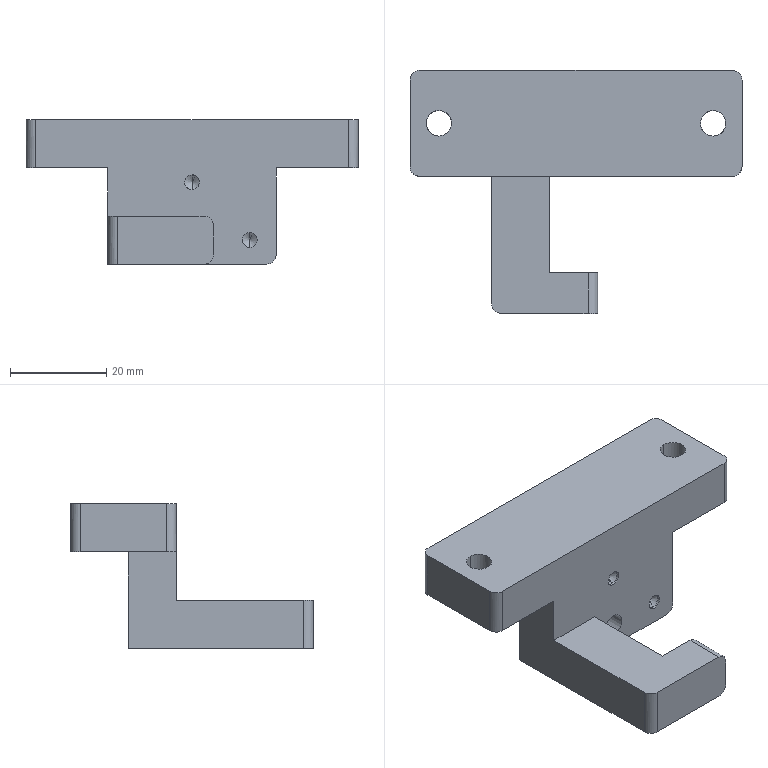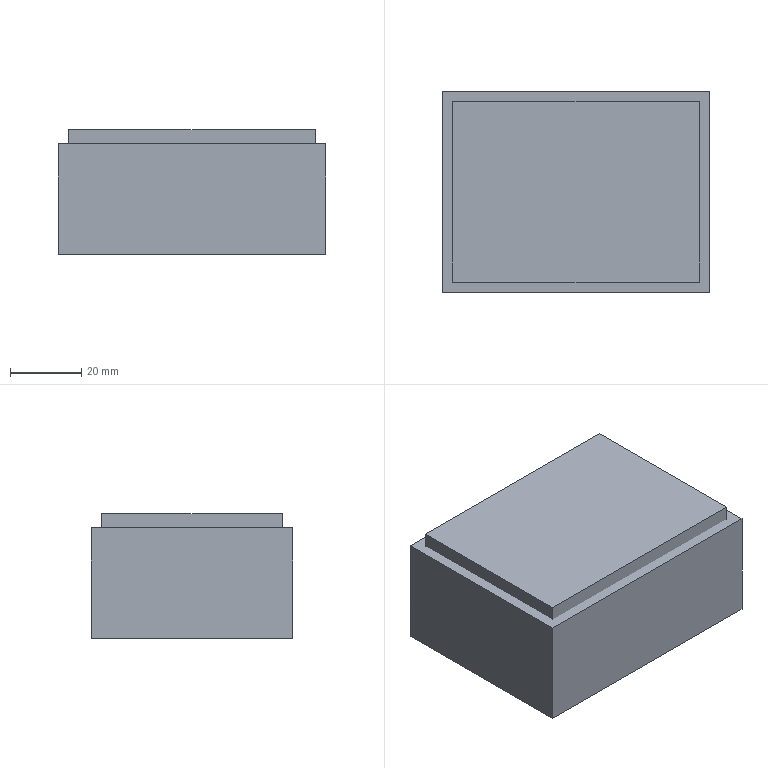CAM job | NX | 3+2 milling, drilling | part box 69 x 50.5 x 30 mm | stock box 75 x 56.5 x 35 mm
Tools:
number,name,description,diameter,corner_radius,flute_length,length,flutes
19,D80,Milling Tool-5 Parameters,80.0,0.0,50.0,75.0,2
15,D10,Milling Tool-5 Parameters,10.0,0.0,50.0,75.0,2
14,D10JING,Milling Tool-5 Parameters,10.0,0.0,50.0,75.0,2
12,D6,Milling Tool-5 Parameters,6.0,0.0,50.0,75.0,2
3,D3,Milling Tool-5 Parameters,3.0,0.0,50.0,75.0,2
1,D6A45,Milling Tool-5 Parameters,6.0,0.0,50.0,75.0,2
2,2.5ZT,Drilling Tool,2.0,0.0,35.0,50.0,2
16,4.8ZT,Drilling Tool,4.8,0.0,35.0,50.0,2
17,5.0JD,Milling Tool-5 Parameters,5.0,0.0,30.0,30.0,4
Operations:
program,operation,operation_type,tool,method,geometry_group,spindle_rpm,surface_speed,feed_per_tooth,feed_cut,feed_plunge,cut_length_mm,path_length_mm,cut_time_min,machine_time_min
1,FLOOR_WALL,VolumeBased25DMillingOperation,D80,METHOD,A,6500.0,1633.0,0.1154,1500.0,100.0,167.0,221.0,0.1113,0.1167
1,CAVITY_MILL,CavityMilling,D10,METHOD,A,9500.0,298.0,0.1579,3000.0,1000.0,24552.14,25216.206,8.38,8.446
1,ZLEVEL_PROFILE_1,ZLevelMilling,D10JING,METHOD,A,9500.0,298.0,0.0789,1500.0,1000.0,847.836,949.836,0.5666,0.5768
1,FLOOR_WALL_1_COPY,VolumeBased25DMillingOperation,D6,METHOD,A,9500.0,179.0,0.0632,1200.0,100.0,309.856,422.913,0.2582,0.2695
1,CAVITY_MILL_COPY,CavityMilling,D6,METHOD,A,9500.0,179.0,0.0632,1200.0,1000.0,415.338,936.871,0.3619,0.414
1,ZLEVEL_PROFILE_1_COPY,ZLevelMilling,D6,METHOD,A,9500.0,179.0,0.1579,3000.0,1000.0,930.279,1029.284,0.3121,0.322
1,HOLE_MILLING,CylinderMilling,D3,METHOD,A,9500.0,89.0,0.0579,1100.0,100.0,780.662,976.662,0.7097,0.7293
1,PLANAR_MILL_COPY,PlanarMilling,D6A45,METHOD,A,9500.0,179.0,0.0658,1250.0,100.0,221.496,463.929,0.1772,0.2014
2,FLOOR_WALL_COPY,VolumeBased25DMillingOperation,D80,METHOD,B,6500.0,1633.0,0.1154,1500.0,100.0,805.0,1675.001,0.5367,0.6237
2,FLOOR_WALL_1_COPY_1,VolumeBased25DMillingOperation,D10,METHOD,B,9500.0,298.0,0.1842,3500.0,100.0,9424.944,9662.171,2.693,2.717
2,FLOOR_WALL_1_COPY_COPY_1_COPY,VolumeBased25DMillingOperation,D10JING,METHOD,B,9500.0,179.0,0.0632,1200.0,100.0,554.072,679.16,0.4617,0.4742
2,ZLEVEL_PROFILE_1_COPY_COPY,ZLevelMilling,D6,METHOD,B,9500.0,179.0,0.1579,3000.0,1000.0,1957.418,2148.093,0.6584,0.6775
2,PLANAR_MILL_COPY_COPY,PlanarMilling,D6A45,METHOD,B,9500.0,179.0,0.0658,1250.0,100.0,176.118,235.118,0.1409,0.1468
2,PLANAR_MILL_COPY_COPY_COPY,PlanarMilling,D6A45,METHOD,B,9500.0,179.0,0.0658,1250.0,100.0,184.881,511.758,0.1479,0.1806
3,DRILLING,Operation,D6A45,METHOD,C,9500.0,179.0,0.0132,250.0,0.0,12.0,128.895,0.048,0.0597
3,DRILLING_COPY_COPY_COPY,Operation,2.5ZT,METHOD,C,2000.0,12.0,0.025,100.0,0.0,22.502,141.491,0.225,0.2369
3,DRILLING_COPY_COPY_COPY_COPY,Operation,4.8ZT,METHOD,C,2000.0,12.0,0.025,100.0,0.0,40.442,164.884,0.4044,0.4169
3,DRILLING_COPY_COPY_COPY_COPY_COPY,Operation,5.0JD,METHOD,C,1000.0,15.0,0.0088,35.0,0.0,39.0,162.0,1.114,1.127